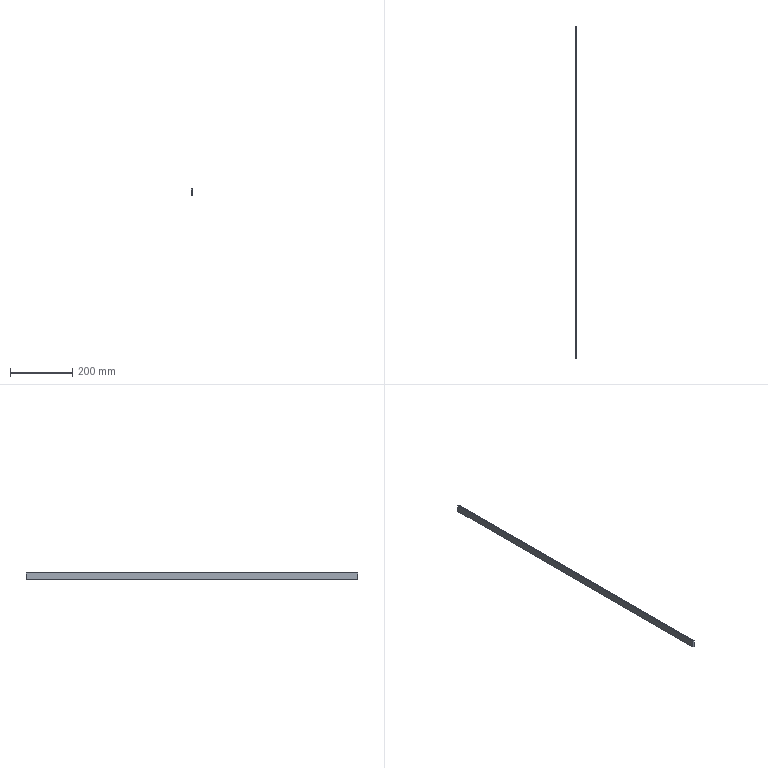Part | NX | features solid 2 | 1 solid | 13 faces | box 6 x 1071 x 24 mm | volume 148945 mm3 | plane 8 | cylinder 5 | commonest cylinder face diameters 1 x2 0.5 x1 2 x1 4 x1
STEP:
#1=CARTESIAN_POINT('',(-15.5,1078.1,-1003.01));
#2=VERTEX_POINT('',#1);
#3=CARTESIAN_POINT('',(-15.833,1078.1,-1003.481));
#4=VERTEX_POINT('',#3);
#5=CARTESIAN_POINT('',(-16.,1078.1,-1003.01));
#6=DIRECTION('',(0.,1.,0.));
#7=DIRECTION('',(1.,0.,0.));
#8=AXIS2_PLACEMENT_3D('',#5,#6,#7);
#9=CIRCLE('',#8,0.5);
#10=EDGE_CURVE('',#2,#4,#9,.T.);
#11=ORIENTED_EDGE('',*,*,#10,.F.);
#12=CARTESIAN_POINT('',(-15.5,1078.1,-1002.01));
#13=VERTEX_POINT('',#12);
#14=CARTESIAN_POINT('',(-15.5,1078.1,-1003.01));
#15=DIRECTION('',(0.,0.,1.));
#16=VECTOR('',#15,1000.);
#17=LINE('',#14,#16);
#18=EDGE_CURVE('',#2,#13,#17,.T.);
#19=ORIENTED_EDGE('',*,*,#18,.T.);
#20=CARTESIAN_POINT('',(-15.,1078.1,-1001.51));
#21=VERTEX_POINT('',#20);
#22=CARTESIAN_POINT('',(-15.,1078.1,-1002.01));
#23=DIRECTION('',(0.,-1.,0.));
#24=DIRECTION('',(0.,0.,1.));
#25=AXIS2_PLACEMENT_3D('',#22,#23,#24);
#26=CIRCLE('',#25,0.5);
#27=EDGE_CURVE('',#21,#13,#26,.T.);
#28=ORIENTED_EDGE('',*,*,#27,.F.);
#29=CARTESIAN_POINT('',(-13.578,1078.1,-1001.51));
#30=VERTEX_POINT('',#29);
#31=CARTESIAN_POINT('',(-15.,1078.1,-1001.51));
#32=DIRECTION('',(1.,0.,0.));
#33=VECTOR('',#32,1000.);
#34=LINE('',#31,#33);
#35=EDGE_CURVE('',#21,#30,#34,.T.);
#36=ORIENTED_EDGE('',*,*,#35,.T.);
#37=CARTESIAN_POINT('',(-12.164,1078.1,-1002.096));
#38=VERTEX_POINT('',#37);
#39=CARTESIAN_POINT('',(-13.578,1078.1,-1003.51));
#40=DIRECTION('',(0.,-1.,0.));
#41=DIRECTION('',(0.7071,0.,0.7071));
#42=AXIS2_PLACEMENT_3D('',#39,#40,#41);
#43=CIRCLE('',#42,2.);
#44=EDGE_CURVE('',#38,#30,#43,.T.);
#45=ORIENTED_EDGE('',*,*,#44,.F.);
#46=CARTESIAN_POINT('',(-10.293,1078.1,-1003.967));
#47=VERTEX_POINT('',#46);
#48=CARTESIAN_POINT('',(-10.293,1078.1,-1003.967));
#49=DIRECTION('',(-0.7071,0.,0.7071));
#50=VECTOR('',#49,1000.);
#51=LINE('',#48,#50);
#52=EDGE_CURVE('',#47,#38,#51,.T.);
#53=ORIENTED_EDGE('',*,*,#52,.F.);
#54=CARTESIAN_POINT('',(-10.,1078.1,-1004.674));
#55=VERTEX_POINT('',#54);
#56=CARTESIAN_POINT('',(-11.,1078.1,-1004.674));
#57=DIRECTION('',(0.,-1.,0.));
#58=DIRECTION('',(1.,0.,0.));
#59=AXIS2_PLACEMENT_3D('',#56,#57,#58);
#60=CIRCLE('',#59,1.);
#61=EDGE_CURVE('',#55,#47,#60,.T.);
#62=ORIENTED_EDGE('',*,*,#61,.F.);
#63=CARTESIAN_POINT('',(-10.,1078.1,-1025.51));
#64=VERTEX_POINT('',#63);
#65=CARTESIAN_POINT('',(-10.,1078.1,-1004.674));
#66=DIRECTION('',(0.,0.,-1.));
#67=VECTOR('',#66,1000.);
#68=LINE('',#65,#67);
#69=EDGE_CURVE('',#55,#64,#68,.T.);
#70=ORIENTED_EDGE('',*,*,#69,.T.);
#71=CARTESIAN_POINT('',(-16.,1078.1,-1025.51));
#72=VERTEX_POINT('',#71);
#73=CARTESIAN_POINT('',(-10.,1078.1,-1025.51));
#74=DIRECTION('',(-1.,0.,0.));
#75=VECTOR('',#74,1000.);
#76=LINE('',#73,#75);
#77=EDGE_CURVE('',#64,#72,#76,.T.);
#78=ORIENTED_EDGE('',*,*,#77,.T.);
#79=CARTESIAN_POINT('',(-16.,1078.1,-1003.717));
#80=VERTEX_POINT('',#79);
#81=CARTESIAN_POINT('',(-16.,1078.1,-1025.51));
#82=DIRECTION('',(0.,0.,1.));
#83=VECTOR('',#82,1000.);
#84=LINE('',#81,#83);
#85=EDGE_CURVE('',#72,#80,#84,.T.);
#86=ORIENTED_EDGE('',*,*,#85,.T.);
#87=CARTESIAN_POINT('',(-15.75,1078.1,-1003.717));
#88=DIRECTION('',(0.,-1.,0.));
#89=DIRECTION('',(-0.3333,0.,0.9428));
#90=AXIS2_PLACEMENT_3D('',#87,#88,#89);
#91=CIRCLE('',#90,0.25);
#92=EDGE_CURVE('',#4,#80,#91,.T.);
#93=ORIENTED_EDGE('',*,*,#92,.F.);
#94=EDGE_LOOP('',(#11,#19,#28,#36,#45,#53,#62,#70,#78,#86,#93));
#95=FACE_BOUND('',#94,.T.);
#96=CARTESIAN_POINT('',(-13.,1078.1,-1013.51));
#97=DIRECTION('',(0.,-1.,0.));
#98=DIRECTION('',(-1.,0.,0.));
#99=AXIS2_PLACEMENT_3D('',#96,#97,#98);
#100=PLANE('',#99);
#101=ADVANCED_FACE('',(#95),#100,.F.);
#102=CARTESIAN_POINT('',(-16.,7.35,-1003.717));
#103=VERTEX_POINT('',#102);
#104=CARTESIAN_POINT('',(-16.,7.35,-1003.717));
#105=DIRECTION('',(0.,1.,0.));
#106=VECTOR('',#105,1000.);
#107=LINE('',#104,#106);
#108=EDGE_CURVE('',#103,#80,#107,.T.);
#109=ORIENTED_EDGE('',*,*,#108,.F.);
#110=CARTESIAN_POINT('',(-15.833,7.35,-1003.481));
#111=VERTEX_POINT('',#110);
#112=CARTESIAN_POINT('',(-15.75,7.35,-1003.717));
#113=DIRECTION('',(0.,1.,0.));
#114=DIRECTION('',(-1.,0.,0.));
#115=AXIS2_PLACEMENT_3D('',#112,#113,#114);
#116=CIRCLE('',#115,0.25);
#117=EDGE_CURVE('',#103,#111,#116,.T.);
#118=ORIENTED_EDGE('',*,*,#117,.T.);
#119=CARTESIAN_POINT('',(-15.833,1078.1,-1003.481));
#120=DIRECTION('',(0.,-1.,0.));
#121=VECTOR('',#120,1000.);
#122=LINE('',#119,#121);
#123=EDGE_CURVE('',#4,#111,#122,.T.);
#124=ORIENTED_EDGE('',*,*,#123,.F.);
#125=ORIENTED_EDGE('',*,*,#92,.T.);
#126=EDGE_LOOP('',(#109,#118,#124,#125));
#127=FACE_BOUND('',#126,.T.);
#128=CARTESIAN_POINT('',(-15.75,-1388.48,-1003.717));
#129=DIRECTION('',(0.,1.,0.));
#130=DIRECTION('',(1.,0.,0.));
#131=AXIS2_PLACEMENT_3D('',#128,#129,#130);
#132=CYLINDRICAL_SURFACE('',#131,0.25);
#133=ADVANCED_FACE('',(#127),#132,.T.);
#134=CARTESIAN_POINT('',(-15.5,7.35,-1003.01));
#135=VERTEX_POINT('',#134);
#136=CARTESIAN_POINT('',(-16.,7.35,-1003.01));
#137=DIRECTION('',(0.,-1.,0.));
#138=DIRECTION('',(0.3333,0.,-0.9428));
#139=AXIS2_PLACEMENT_3D('',#136,#137,#138);
#140=CIRCLE('',#139,0.5);
#141=EDGE_CURVE('',#111,#135,#140,.T.);
#142=ORIENTED_EDGE('',*,*,#141,.T.);
#143=CARTESIAN_POINT('',(-15.5,1078.1,-1003.01));
#144=DIRECTION('',(0.,-1.,0.));
#145=VECTOR('',#144,1000.);
#146=LINE('',#143,#145);
#147=EDGE_CURVE('',#2,#135,#146,.T.);
#148=ORIENTED_EDGE('',*,*,#147,.F.);
#149=ORIENTED_EDGE('',*,*,#10,.T.);
#150=ORIENTED_EDGE('',*,*,#123,.T.);
#151=EDGE_LOOP('',(#142,#148,#149,#150));
#152=FACE_BOUND('',#151,.T.);
#153=CARTESIAN_POINT('',(-16.,-1388.48,-1003.01));
#154=DIRECTION('',(0.,1.,0.));
#155=DIRECTION('',(-1.,0.,0.));
#156=AXIS2_PLACEMENT_3D('',#153,#154,#155);
#157=CYLINDRICAL_SURFACE('',#156,0.5);
#158=ADVANCED_FACE('',(#152),#157,.F.);
#159=ORIENTED_EDGE('',*,*,#18,.F.);
#160=ORIENTED_EDGE('',*,*,#147,.T.);
#161=CARTESIAN_POINT('',(-15.5,7.35,-1002.01));
#162=VERTEX_POINT('',#161);
#163=CARTESIAN_POINT('',(-15.5,7.35,-1003.01));
#164=DIRECTION('',(0.,0.,1.));
#165=VECTOR('',#164,1000.);
#166=LINE('',#163,#165);
#167=EDGE_CURVE('',#135,#162,#166,.T.);
#168=ORIENTED_EDGE('',*,*,#167,.T.);
#169=CARTESIAN_POINT('',(-15.5,7.35,-1002.01));
#170=DIRECTION('',(0.,1.,0.));
#171=VECTOR('',#170,1000.);
#172=LINE('',#169,#171);
#173=EDGE_CURVE('',#162,#13,#172,.T.);
#174=ORIENTED_EDGE('',*,*,#173,.T.);
#175=EDGE_LOOP('',(#159,#160,#168,#174));
#176=FACE_BOUND('',#175,.T.);
#177=CARTESIAN_POINT('',(-15.5,1078.1,-1013.51));
#178=DIRECTION('',(-1.,0.,0.));
#179=DIRECTION('',(0.,-1.,0.));
#180=AXIS2_PLACEMENT_3D('',#177,#178,#179);
#181=PLANE('',#180);
#182=ADVANCED_FACE('',(#176),#181,.T.);
#183=CARTESIAN_POINT('',(-15.,7.35,-1001.51));
#184=VERTEX_POINT('',#183);
#185=CARTESIAN_POINT('',(-15.,1078.1,-1001.51));
#186=DIRECTION('',(0.,-1.,0.));
#187=VECTOR('',#186,1000.);
#188=LINE('',#185,#187);
#189=EDGE_CURVE('',#21,#184,#188,.T.);
#190=ORIENTED_EDGE('',*,*,#189,.F.);
#191=ORIENTED_EDGE('',*,*,#27,.T.);
#192=ORIENTED_EDGE('',*,*,#173,.F.);
#193=CARTESIAN_POINT('',(-15.,7.35,-1002.01));
#194=DIRECTION('',(0.,1.,0.));
#195=DIRECTION('',(-1.,0.,0.));
#196=AXIS2_PLACEMENT_3D('',#193,#194,#195);
#197=CIRCLE('',#196,0.5);
#198=EDGE_CURVE('',#162,#184,#197,.T.);
#199=ORIENTED_EDGE('',*,*,#198,.T.);
#200=EDGE_LOOP('',(#190,#191,#192,#199));
#201=FACE_BOUND('',#200,.T.);
#202=CARTESIAN_POINT('',(-15.,2473.93,-1002.01));
#203=DIRECTION('',(0.,-1.,0.));
#204=DIRECTION('',(0.,0.,-1.));
#205=AXIS2_PLACEMENT_3D('',#202,#203,#204);
#206=CYLINDRICAL_SURFACE('',#205,0.5);
#207=ADVANCED_FACE('',(#201),#206,.T.);
#208=CARTESIAN_POINT('',(-16.,7.35,-1025.51));
#209=VERTEX_POINT('',#208);
#210=CARTESIAN_POINT('',(-16.,7.35,-1025.51));
#211=DIRECTION('',(0.,0.,1.));
#212=VECTOR('',#211,1000.);
#213=LINE('',#210,#212);
#214=EDGE_CURVE('',#209,#103,#213,.T.);
#215=ORIENTED_EDGE('',*,*,#214,.F.);
#216=CARTESIAN_POINT('',(-10.,7.35,-1025.51));
#217=VERTEX_POINT('',#216);
#218=CARTESIAN_POINT('',(-10.,7.35,-1025.51));
#219=DIRECTION('',(-1.,0.,0.));
#220=VECTOR('',#219,1000.);
#221=LINE('',#218,#220);
#222=EDGE_CURVE('',#217,#209,#221,.T.);
#223=ORIENTED_EDGE('',*,*,#222,.F.);
#224=CARTESIAN_POINT('',(-10.,7.35,-1004.674));
#225=VERTEX_POINT('',#224);
#226=CARTESIAN_POINT('',(-10.,7.35,-1004.674));
#227=DIRECTION('',(0.,0.,-1.));
#228=VECTOR('',#227,1000.);
#229=LINE('',#226,#228);
#230=EDGE_CURVE('',#225,#217,#229,.T.);
#231=ORIENTED_EDGE('',*,*,#230,.F.);
#232=CARTESIAN_POINT('',(-10.293,7.35,-1003.967));
#233=VERTEX_POINT('',#232);
#234=CARTESIAN_POINT('',(-11.,7.35,-1004.674));
#235=DIRECTION('',(0.,1.,0.));
#236=DIRECTION('',(0.7071,0.,0.7071));
#237=AXIS2_PLACEMENT_3D('',#234,#235,#236);
#238=CIRCLE('',#237,1.);
#239=EDGE_CURVE('',#233,#225,#238,.T.);
#240=ORIENTED_EDGE('',*,*,#239,.F.);
#241=CARTESIAN_POINT('',(-12.164,7.35,-1002.096));
#242=VERTEX_POINT('',#241);
#243=CARTESIAN_POINT('',(-12.164,7.35,-1002.096));
#244=DIRECTION('',(0.7071,0.,-0.7071));
#245=VECTOR('',#244,1000.);
#246=LINE('',#243,#245);
#247=EDGE_CURVE('',#242,#233,#246,.T.);
#248=ORIENTED_EDGE('',*,*,#247,.F.);
#249=CARTESIAN_POINT('',(-13.578,7.35,-1001.51));
#250=VERTEX_POINT('',#249);
#251=CARTESIAN_POINT('',(-13.578,7.35,-1003.51));
#252=DIRECTION('',(0.,1.,0.));
#253=DIRECTION('',(0.,0.,1.));
#254=AXIS2_PLACEMENT_3D('',#251,#252,#253);
#255=CIRCLE('',#254,2.);
#256=EDGE_CURVE('',#250,#242,#255,.T.);
#257=ORIENTED_EDGE('',*,*,#256,.F.);
#258=CARTESIAN_POINT('',(-15.,7.35,-1001.51));
#259=DIRECTION('',(1.,0.,0.));
#260=VECTOR('',#259,1000.);
#261=LINE('',#258,#260);
#262=EDGE_CURVE('',#184,#250,#261,.T.);
#263=ORIENTED_EDGE('',*,*,#262,.F.);
#264=ORIENTED_EDGE('',*,*,#198,.F.);
#265=ORIENTED_EDGE('',*,*,#167,.F.);
#266=ORIENTED_EDGE('',*,*,#141,.F.);
#267=ORIENTED_EDGE('',*,*,#117,.F.);
#268=EDGE_LOOP('',(#215,#223,#231,#240,#248,#257,#263,#264,#265,#266,#267));
#269=FACE_BOUND('',#268,.T.);
#270=CARTESIAN_POINT('',(-13.,7.35,-1013.51));
#271=DIRECTION('',(0.,-1.,0.));
#272=DIRECTION('',(-1.,0.,0.));
#273=AXIS2_PLACEMENT_3D('',#270,#271,#272);
#274=PLANE('',#273);
#275=ADVANCED_FACE('',(#269),#274,.T.);
#276=ORIENTED_EDGE('',*,*,#262,.T.);
#277=CARTESIAN_POINT('',(-13.578,7.35,-1001.51));
#278=DIRECTION('',(0.,1.,0.));
#279=VECTOR('',#278,1000.);
#280=LINE('',#277,#279);
#281=EDGE_CURVE('',#250,#30,#280,.T.);
#282=ORIENTED_EDGE('',*,*,#281,.T.);
#283=ORIENTED_EDGE('',*,*,#35,.F.);
#284=ORIENTED_EDGE('',*,*,#189,.T.);
#285=EDGE_LOOP('',(#276,#282,#283,#284));
#286=FACE_BOUND('',#285,.T.);
#287=CARTESIAN_POINT('',(-10.,1078.1,-1001.51));
#288=DIRECTION('',(0.,0.,1.));
#289=DIRECTION('',(1.,0.,0.));
#290=AXIS2_PLACEMENT_3D('',#287,#288,#289);
#291=PLANE('',#290);
#292=ADVANCED_FACE('',(#286),#291,.T.);
#293=ORIENTED_EDGE('',*,*,#281,.F.);
#294=ORIENTED_EDGE('',*,*,#256,.T.);
#295=CARTESIAN_POINT('',(-12.164,1078.1,-1002.096));
#296=DIRECTION('',(0.,-1.,0.));
#297=VECTOR('',#296,1000.);
#298=LINE('',#295,#297);
#299=EDGE_CURVE('',#38,#242,#298,.T.);
#300=ORIENTED_EDGE('',*,*,#299,.F.);
#301=ORIENTED_EDGE('',*,*,#44,.T.);
#302=EDGE_LOOP('',(#293,#294,#300,#301));
#303=FACE_BOUND('',#302,.T.);
#304=CARTESIAN_POINT('',(-13.578,-1388.48,-1003.51));
#305=DIRECTION('',(0.,1.,0.));
#306=DIRECTION('',(0.,0.,-1.));
#307=AXIS2_PLACEMENT_3D('',#304,#305,#306);
#308=CYLINDRICAL_SURFACE('',#307,2.);
#309=ADVANCED_FACE('',(#303),#308,.T.);
#310=ORIENTED_EDGE('',*,*,#247,.T.);
#311=CARTESIAN_POINT('',(-10.293,7.35,-1003.967));
#312=DIRECTION('',(0.,1.,0.));
#313=VECTOR('',#312,1000.);
#314=LINE('',#311,#313);
#315=EDGE_CURVE('',#233,#47,#314,.T.);
#316=ORIENTED_EDGE('',*,*,#315,.T.);
#317=ORIENTED_EDGE('',*,*,#52,.T.);
#318=ORIENTED_EDGE('',*,*,#299,.T.);
#319=EDGE_LOOP('',(#310,#316,#317,#318));
#320=FACE_BOUND('',#319,.T.);
#321=CARTESIAN_POINT('',(-11.375,542.725,-1002.885));
#322=DIRECTION('',(0.7071,0.,0.7071));
#323=DIRECTION('',(-0.7071,0.,0.7071));
#324=AXIS2_PLACEMENT_3D('',#321,#322,#323);
#325=PLANE('',#324);
#326=ADVANCED_FACE('',(#320),#325,.T.);
#327=CARTESIAN_POINT('',(-10.,1078.1,-1004.674));
#328=DIRECTION('',(0.,-1.,0.));
#329=VECTOR('',#328,1000.);
#330=LINE('',#327,#329);
#331=EDGE_CURVE('',#55,#225,#330,.T.);
#332=ORIENTED_EDGE('',*,*,#331,.F.);
#333=ORIENTED_EDGE('',*,*,#61,.T.);
#334=ORIENTED_EDGE('',*,*,#315,.F.);
#335=ORIENTED_EDGE('',*,*,#239,.T.);
#336=EDGE_LOOP('',(#332,#333,#334,#335));
#337=FACE_BOUND('',#336,.T.);
#338=CARTESIAN_POINT('',(-11.,2473.93,-1004.674));
#339=DIRECTION('',(0.,-1.,0.));
#340=DIRECTION('',(-1.,0.,0.));
#341=AXIS2_PLACEMENT_3D('',#338,#339,#340);
#342=CYLINDRICAL_SURFACE('',#341,1.);
#343=ADVANCED_FACE('',(#337),#342,.T.);
#344=ORIENTED_EDGE('',*,*,#230,.T.);
#345=CARTESIAN_POINT('',(-10.,7.35,-1025.51));
#346=DIRECTION('',(0.,1.,0.));
#347=VECTOR('',#346,1000.);
#348=LINE('',#345,#347);
#349=EDGE_CURVE('',#217,#64,#348,.T.);
#350=ORIENTED_EDGE('',*,*,#349,.T.);
#351=ORIENTED_EDGE('',*,*,#69,.F.);
#352=ORIENTED_EDGE('',*,*,#331,.T.);
#353=EDGE_LOOP('',(#344,#350,#351,#352));
#354=FACE_BOUND('',#353,.T.);
#355=CARTESIAN_POINT('',(-10.,1078.1,-1025.51));
#356=DIRECTION('',(1.,0.,0.));
#357=DIRECTION('',(0.,0.,-1.));
#358=AXIS2_PLACEMENT_3D('',#355,#356,#357);
#359=PLANE('',#358);
#360=ADVANCED_FACE('',(#354),#359,.T.);
#361=ORIENTED_EDGE('',*,*,#349,.F.);
#362=ORIENTED_EDGE('',*,*,#222,.T.);
#363=CARTESIAN_POINT('',(-16.,7.35,-1025.51));
#364=DIRECTION('',(0.,1.,0.));
#365=VECTOR('',#364,1000.);
#366=LINE('',#363,#365);
#367=EDGE_CURVE('',#209,#72,#366,.T.);
#368=ORIENTED_EDGE('',*,*,#367,.T.);
#369=ORIENTED_EDGE('',*,*,#77,.F.);
#370=EDGE_LOOP('',(#361,#362,#368,#369));
#371=FACE_BOUND('',#370,.T.);
#372=CARTESIAN_POINT('',(-16.,1078.1,-1025.51));
#373=DIRECTION('',(0.,0.,-1.));
#374=DIRECTION('',(-1.,0.,0.));
#375=AXIS2_PLACEMENT_3D('',#372,#373,#374);
#376=PLANE('',#375);
#377=ADVANCED_FACE('',(#371),#376,.T.);
#378=ORIENTED_EDGE('',*,*,#85,.F.);
#379=ORIENTED_EDGE('',*,*,#367,.F.);
#380=ORIENTED_EDGE('',*,*,#214,.T.);
#381=ORIENTED_EDGE('',*,*,#108,.T.);
#382=EDGE_LOOP('',(#378,#379,#380,#381));
#383=FACE_BOUND('',#382,.T.);
#384=CARTESIAN_POINT('',(-16.,1078.1,-1001.51));
#385=DIRECTION('',(-1.,0.,0.));
#386=DIRECTION('',(0.,0.,1.));
#387=AXIS2_PLACEMENT_3D('',#384,#385,#386);
#388=PLANE('',#387);
#389=ADVANCED_FACE('',(#383),#388,.T.);
#390=CLOSED_SHELL('',(#101,#133,#158,#182,#207,#275,#292,#309,#326,#343,#360,#377,#389));
#391=MANIFOLD_SOLID_BREP('',#390);
#392=(LENGTH_UNIT()NAMED_UNIT(*)SI_UNIT(.MILLI.,.METRE.));
#393=UNCERTAINTY_MEASURE_WITH_UNIT(LENGTH_MEASURE(0.00001),#392,'','');
#394=(NAMED_UNIT(*)PLANE_ANGLE_UNIT()SI_UNIT($,.RADIAN.));
#395=(NAMED_UNIT(*)SI_UNIT($,.STERADIAN.)SOLID_ANGLE_UNIT());
#396=(GEOMETRIC_REPRESENTATION_CONTEXT(3)GLOBAL_UNCERTAINTY_ASSIGNED_CONTEXT((#393))GLOBAL_UNIT_ASSIGNED_CONTEXT((#392,#394,#395))REPRESENTATION_CONTEXT('',''));
#397=ADVANCED_BREP_SHAPE_REPRESENTATION('',(#391),#396);